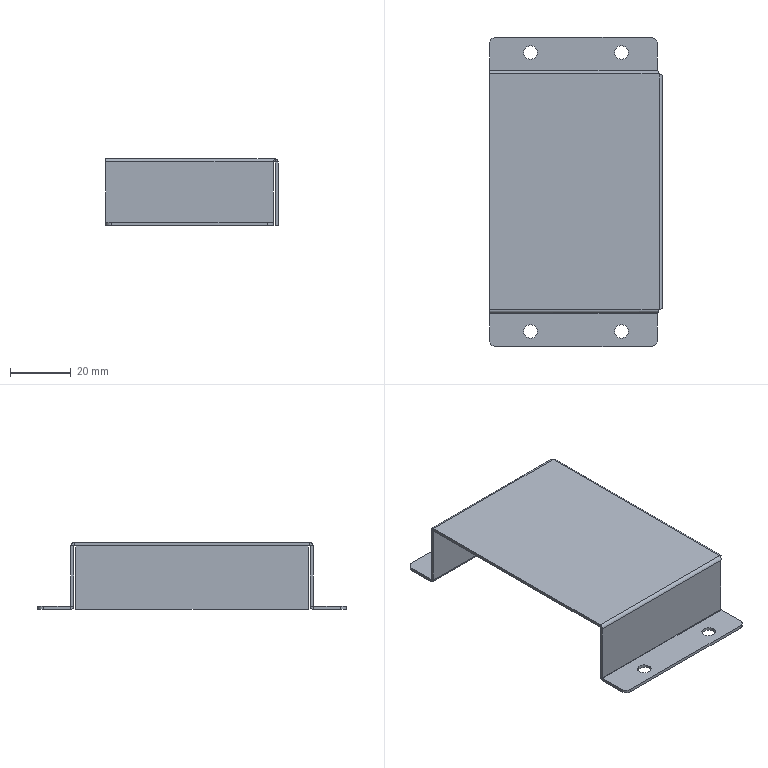Part | STEP file | 1 solid | 58 faces | box 57 x 102 x 22 mm | volume 9559 mm3 | plane 32 | cylinder 22 | spline 4 | commonest cylinder face diameters 4.5 x8 0.2 x5 2.2 x5 4 x4